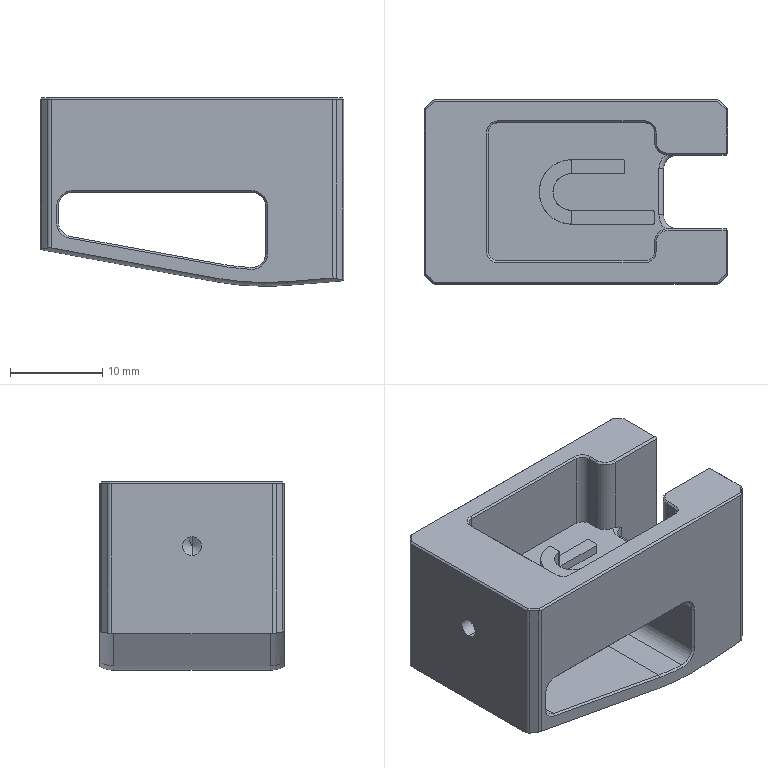NC program | NX | posted with a generic post | part box 33 x 20 x 20.478 mm
Lines 3457 to 5321 of 8500, first 1748 of 1863 lines:
(ZLEVEL_PROFILE_COPY , TOOL : D3)
N6882 T16 M6
N6884 G54
N6886 G17 G0 G90 X13.266 Y1.9 B0. C0. S9500 M3
N6888 G43 Z30. H16
N6890 Z0.301
N6892 G94 G1 Z-0.199 F1000.
N6894 X13.006 Y2.35
N6896 G3 X12.746 Y2.5 R0.3
N6898 G1 X11.
N6900 Y0.748
N6902 G3 X11.15 Y0.488 R0.3
N6904 G1 X11.6 Y0.228
N6906 Z0.301
N6908 G0 X13.266 Y1.9 Z0.102
N6910 G1 Z-0.398
N6912 X13.006 Y2.35
N6914 G3 X12.746 Y2.5 R0.3
N6916 G1 X11.
N6918 Y0.748
N6920 G3 X11.15 Y0.488 R0.3
N6922 G1 X11.6 Y0.228
N6924 Z0.102
N6926 G0 X13.266 Y1.9 Z-0.096
N6928 G1 Z-0.596
N6930 X13.006 Y2.35
N6932 G3 X12.746 Y2.5 R0.3
N6934 G1 X11.
N6936 Y0.748
N6938 G3 X11.15 Y0.488 R0.3
N6940 G1 X11.6 Y0.228
N6942 Z-0.096
N6944 G0 X13.266 Y1.9 Z-0.295
N6946 G1 Z-0.795
N6948 X13.006 Y2.35
N6950 G3 X12.746 Y2.5 R0.3
N6952 G1 X11.
N6954 Y0.748
N6956 G3 X11.15 Y0.488 R0.3
N6958 G1 X11.6 Y0.228
N6960 Z-0.295
N6962 G0 X13.266 Y1.9 Z-0.494
N6964 G1 Z-0.994
N6966 X13.006 Y2.35
N6968 G3 X12.746 Y2.5 R0.3
N6970 G1 X11.
N6972 Y0.748
N6974 G3 X11.15 Y0.488 R0.3
N6976 G1 X11.6 Y0.228
N6978 Z-0.494
N6980 G0 X13.266 Y1.9 Z-0.693
N6982 G1 Z-1.193
N6984 X13.006 Y2.35
N6986 G3 X12.746 Y2.5 R0.3
N6988 G1 X11.
N6990 Y0.748
N6992 G3 X11.15 Y0.488 R0.3
N6994 G1 X11.6 Y0.228
N6996 Z-0.693
N6998 G0 X13.266 Y1.9 Z-0.892
N7000 G1 Z-1.392
N7002 X13.006 Y2.35
N7004 G3 X12.746 Y2.5 R0.3
N7006 G1 X11.
N7008 Y0.748
N7010 G3 X11.15 Y0.488 R0.3
N7012 G1 X11.6 Y0.228
N7014 Z-0.892
N7016 G0 X13.266 Y1.9 Z-1.091
N7018 G1 Z-1.591
N7020 X13.006 Y2.35
N7022 G3 X12.746 Y2.5 R0.3
N7024 G1 X11.
N7026 Y0.748
N7028 G3 X11.15 Y0.488 R0.3
N7030 G1 X11.6 Y0.228
N7032 Z-1.091
N7034 G0 X13.266 Y1.9 Z-1.289
N7036 G1 Z-1.789
N7038 X13.006 Y2.35
N7040 G3 X12.746 Y2.5 R0.3
N7042 G1 X11.
N7044 Y0.748
N7046 G3 X11.15 Y0.488 R0.3
N7048 G1 X11.6 Y0.228
N7050 Z-1.289
N7052 G0 X13.266 Y1.9 Z-1.488
N7054 G1 Z-1.988
N7056 X13.006 Y2.35
N7058 G3 X12.746 Y2.5 R0.3
N7060 G1 X11.
N7062 Y0.748
N7064 G3 X11.15 Y0.488 R0.3
N7066 G1 X11.6 Y0.228
N7068 Z-1.488
N7070 G0 X13.266 Y1.9 Z-1.687
N7072 G1 Z-2.187
N7074 X13.006 Y2.35
N7076 G3 X12.746 Y2.5 R0.3
N7078 G1 X11.
N7080 Y0.748
N7082 G3 X11.15 Y0.488 R0.3
N7084 G1 X11.6 Y0.228
N7086 Z-1.687
N7088 G0 X13.266 Y1.9 Z-1.886
N7090 G1 Z-2.386
N7092 X13.006 Y2.35
N7094 G3 X12.746 Y2.5 R0.3
N7096 G1 X11.
N7098 Y0.748
N7100 G3 X11.15 Y0.488 R0.3
N7102 G1 X11.6 Y0.228
N7104 Z-1.886
N7106 G0 X13.266 Y1.9 Z-2.085
N7108 G1 Z-2.585
N7110 X13.006 Y2.35
N7112 G3 X12.746 Y2.5 R0.3
N7114 G1 X11.
N7116 Y0.748
N7118 G3 X11.15 Y0.488 R0.3
N7120 G1 X11.6 Y0.228
N7122 Z-2.085
N7124 G0 X13.266 Y1.9 Z-2.283
N7126 G1 Z-2.783
N7128 X13.006 Y2.35
N7130 G3 X12.746 Y2.5 R0.3
N7132 G1 X11.
N7134 Y0.748
N7136 G3 X11.15 Y0.488 R0.3
N7138 G1 X11.6 Y0.228
N7140 Z-2.283
N7142 G0 X13.266 Y1.9 Z-2.482
N7144 G1 Z-2.982
N7146 X13.006 Y2.35
N7148 G3 X12.746 Y2.5 R0.3
N7150 G1 X11.
N7152 Y0.748
N7154 G3 X11.15 Y0.488 R0.3
N7156 G1 X11.6 Y0.228
N7158 Z-2.482
N7160 G0 X13.266 Y1.9 Z-2.681
N7162 G1 Z-3.181
N7164 X13.006 Y2.35
N7166 G3 X12.746 Y2.5 R0.3
N7168 G1 X11.
N7170 Y0.748
N7172 G3 X11.15 Y0.488 R0.3
N7174 G1 X11.6 Y0.228
N7176 Z-2.681
N7178 G0 X13.266 Y1.9 Z-2.88
N7180 G1 Z-3.38
N7182 X13.006 Y2.35
N7184 G3 X12.746 Y2.5 R0.3
N7186 G1 X11.
N7188 Y0.748
N7190 G3 X11.15 Y0.488 R0.3
N7192 G1 X11.6 Y0.228
N7194 Z-2.88
N7196 G0 X13.266 Y1.9 Z-3.079
N7198 G1 Z-3.579
N7200 X13.006 Y2.35
N7202 G3 X12.746 Y2.5 R0.3
N7204 G1 X11.
N7206 Y0.748
N7208 G3 X11.15 Y0.488 R0.3
N7210 G1 X11.6 Y0.228
N7212 Z-3.079
N7214 G0 X13.266 Y1.9 Z-3.278
N7216 G1 Z-3.778
N7218 X13.006 Y2.35
N7220 G3 X12.746 Y2.5 R0.3
N7222 G1 X11.
N7224 Y0.748
N7226 G3 X11.15 Y0.488 R0.3
N7228 G1 X11.6 Y0.228
N7230 Z-3.278
N7232 G0 X13.266 Y1.9 Z-3.476
N7234 G1 Z-3.976
N7236 X13.006 Y2.35
N7238 G3 X12.746 Y2.5 R0.3
N7240 G1 X11.
N7242 Y0.748
N7244 G3 X11.15 Y0.488 R0.3
N7246 G1 X11.6 Y0.228
N7248 Z-3.476
N7250 G0 X13.266 Y1.9 Z-3.675
N7252 G1 Z-4.175
N7254 X13.006 Y2.35
N7256 G3 X12.746 Y2.5 R0.3
N7258 G1 X11.
N7260 Y0.748
N7262 G3 X11.15 Y0.488 R0.3
N7264 G1 X11.6 Y0.228
N7266 Z-3.675
N7268 G0 X13.266 Y1.9 Z-3.874
N7270 G1 Z-4.374
N7272 X13.006 Y2.35
N7274 G3 X12.746 Y2.5 R0.3
N7276 G1 X11.
N7278 Y0.748
N7280 G3 X11.15 Y0.488 R0.3
N7282 G1 X11.6 Y0.228
N7284 Z-3.874
N7286 G0 X13.266 Y1.9 Z-4.073
N7288 G1 Z-4.573
N7290 X13.006 Y2.35
N7292 G3 X12.746 Y2.5 R0.3
N7294 G1 X11.
N7296 Y0.748
N7298 G3 X11.15 Y0.488 R0.3
N7300 G1 X11.6 Y0.228
N7302 Z-4.073
N7304 G0 X13.266 Y1.9 Z-4.272
N7306 G1 Z-4.772
N7308 X13.006 Y2.35
N7310 G3 X12.746 Y2.5 R0.3
N7312 G1 X11.
N7314 Y0.748
N7316 G3 X11.15 Y0.488 R0.3
N7318 G1 X11.6 Y0.228
N7320 Z-4.272
N7322 G0 X13.266 Y1.9 Z-4.47
N7324 G1 Z-4.97
N7326 X13.006 Y2.35
N7328 G3 X12.746 Y2.5 R0.3
N7330 G1 X11.
N7332 Y0.748
N7334 G3 X11.15 Y0.488 R0.3
N7336 G1 X11.6 Y0.228
N7338 Z-4.47
N7340 G0 X13.266 Y1.9 Z-4.669
N7342 G1 Z-5.169
N7344 X13.006 Y2.35
N7346 G3 X12.746 Y2.5 R0.3
N7348 G1 X11.
N7350 Y0.748
N7352 G3 X11.15 Y0.488 R0.3
N7354 G1 X11.6 Y0.228
N7356 Z-4.669
N7358 G0 X13.266 Y1.9 Z-4.868
N7360 G1 Z-5.368
N7362 X13.006 Y2.35
N7364 G3 X12.746 Y2.5 R0.3
N7366 G1 X11.
N7368 Y0.748
N7370 G3 X11.15 Y0.488 R0.3
N7372 G1 X11.6 Y0.228
N7374 Z-4.868
N7376 G0 X13.266 Y1.9 Z-5.067
N7378 G1 Z-5.567
N7380 X13.006 Y2.35
N7382 G3 X12.746 Y2.5 R0.3
N7384 G1 X11.
N7386 Y0.748
N7388 G3 X11.15 Y0.488 R0.3
N7390 G1 X11.6 Y0.228
N7392 Z-5.067
N7394 G0 X13.266 Y1.9 Z-5.266
N7396 G1 Z-5.766
N7398 X13.006 Y2.35
N7400 G3 X12.746 Y2.5 R0.3
N7402 G1 X11.
N7404 Y0.748
N7406 G3 X11.15 Y0.488 R0.3
N7408 G1 X11.6 Y0.228
N7410 Z-5.266
N7412 G0 X13.266 Y1.9 Z-5.465
N7414 G1 Z-5.965
N7416 X13.006 Y2.35
N7418 G3 X12.746 Y2.5 R0.3
N7420 G1 X11.
N7422 Y0.748
N7424 G3 X11.15 Y0.488 R0.3
N7426 G1 X11.6 Y0.228
N7428 Z-5.465
N7430 G0 X13.266 Y1.9 Z-5.663
N7432 G1 Z-6.163
N7434 X13.006 Y2.35
N7436 G3 X12.746 Y2.5 R0.3
N7438 G1 X11.
N7440 Y0.748
N7442 G3 X11.15 Y0.488 R0.3
N7444 G1 X11.6 Y0.228
N7446 Z-5.663
N7448 G0 X13.266 Y1.9 Z-5.862
N7450 G1 Z-6.362
N7452 X13.006 Y2.35
N7454 G3 X12.747 Y2.5 R0.3
N7456 G1 X11.
N7458 Y0.748
N7460 G3 X11.15 Y0.488 R0.3
N7462 G1 X11.6 Y0.228
N7464 Z-5.862
N7466 G0 X13.266 Y1.9 Z-6.061
N7468 G1 Z-6.561
N7470 X13.006 Y2.35
N7472 G3 X12.747 Y2.5 R0.3
N7474 G1 X11.
N7476 Y0.748
N7478 G3 X11.15 Y0.488 R0.3
N7480 G1 X11.6 Y0.228
N7482 Z-6.061
N7484 G0 X13.266 Y1.9 Z-6.26
N7486 G1 Z-6.76
N7488 X13.006 Y2.35
N7490 G3 X12.747 Y2.5 R0.3
N7492 G1 X11.
N7494 Y0.748
N7496 G3 X11.15 Y0.488 R0.3
N7498 G1 X11.6 Y0.228
N7500 Z-6.26
N7502 G0 X13.266 Y1.9 Z-6.459
N7504 G1 Z-6.959
N7506 X13.006 Y2.35
N7508 G3 X12.747 Y2.5 R0.3
N7510 G1 X11.
N7512 Y0.748
N7514 G3 X11.15 Y0.488 R0.3
N7516 G1 X11.6 Y0.228
N7518 Z-6.459
N7520 G0 X13.266 Y1.9 Z-6.657
N7522 G1 Z-7.157
N7524 X13.006 Y2.35
N7526 G3 X12.747 Y2.5 R0.3
N7528 G1 X11.
N7530 Y0.748
N7532 G3 X11.15 Y0.488 R0.3
N7534 G1 X11.6 Y0.228
N7536 Z-6.657
N7538 G0 X13.266 Y1.9 Z-6.856
N7540 G1 Z-7.356
N7542 X13.006 Y2.35
N7544 G3 X12.747 Y2.5 R0.3
N7546 G1 X11.
N7548 Y0.748
N7550 G3 X11.15 Y0.488 R0.3
N7552 G1 X11.6 Y0.228
N7554 Z-6.856
N7556 G0 X13.266 Y1.9 Z-7.055
N7558 G1 Z-7.555
N7560 X13.006 Y2.35
N7562 G3 X12.747 Y2.5 R0.3
N7564 G1 X11.
N7566 Y0.748
N7568 G3 X11.15 Y0.488 R0.3
N7570 G1 X11.6 Y0.228
N7572 Z-7.055
N7574 G0 X13.266 Y1.9 Z-7.254
N7576 G1 Z-7.754
N7578 X13.006 Y2.35
N7580 G3 X12.747 Y2.5 R0.3
N7582 G1 X11.
N7584 Y0.748
N7586 G3 X11.15 Y0.488 R0.3
N7588 G1 X11.6 Y0.228
N7590 Z-7.254
N7592 G0 X13.266 Y1.9 Z-7.453
N7594 G1 Z-7.953
N7596 X13.006 Y2.35
N7598 G3 X12.747 Y2.5 R0.3
N7600 G1 X11.
N7602 Y0.748
N7604 G3 X11.15 Y0.488 R0.3
N7606 G1 X11.6 Y0.228
N7608 Z-7.453
N7610 G0 X13.266 Y1.9 Z-7.652
N7612 G1 Z-8.152
N7614 X13.006 Y2.35
N7616 G3 X12.747 Y2.5 R0.3
N7618 G1 X11.
N7620 Y0.748
N7622 G3 X11.15 Y0.488 R0.3
N7624 G1 X11.6 Y0.228
N7626 Z-7.652
N7628 G0 X13.266 Y1.9 Z-7.85
N7630 G1 Z-8.35
N7632 X13.006 Y2.35
N7634 G3 X12.747 Y2.5 R0.3
N7636 G1 X11.
N7638 Y0.748
N7640 G3 X11.15 Y0.488 R0.3
N7642 G1 X11.6 Y0.228
N7644 Z-7.85
N7646 G0 X13.266 Y1.9 Z-8.049
N7648 G1 Z-8.549
N7650 X13.006 Y2.35
N7652 G3 X12.747 Y2.5 R0.3
N7654 G1 X11.
N7656 Y0.748
N7658 G3 X11.15 Y0.488 R0.3
N7660 G1 X11.6 Y0.228
N7662 Z-8.049
N7664 G0 X13.266 Y1.9 Z-8.248
N7666 G1 Z-8.748
N7668 X13.006 Y2.35
N7670 G3 X12.747 Y2.5 R0.3
N7672 G1 X11.
N7674 Y0.748
N7676 G3 X11.15 Y0.488 R0.3
N7678 G1 X11.6 Y0.228
N7680 Z-8.248
N7682 G0 X13.266 Y1.9 Z-8.447
N7684 G1 Z-8.947
N7686 X13.006 Y2.35
N7688 G3 X12.747 Y2.5 R0.3
N7690 G1 X11.
N7692 Y0.748
N7694 G3 X11.15 Y0.488 R0.3
N7696 G1 X11.6 Y0.228
N7698 Z-8.447
N7700 G0 X13.266 Y1.9 Z-8.646
N7702 G1 Z-9.146
N7704 X13.006 Y2.35
N7706 G3 X12.747 Y2.5 R0.3
N7708 G1 X11.
N7710 Y0.748
N7712 G3 X11.15 Y0.488 R0.3
N7714 G1 X11.6 Y0.228
N7716 Z-8.646
N7718 G0 X13.266 Y1.9 Z-8.844
N7720 G1 Z-9.344
N7722 X13.006 Y2.35
N7724 G3 X12.747 Y2.5 R0.3
N7726 G1 X11.
N7728 Y0.748
N7730 G3 X11.15 Y0.488 R0.3
N7732 G1 X11.6 Y0.228
N7734 Z-8.844
N7736 G0 X13.266 Y1.9 Z-9.043
N7738 G1 Z-9.543
N7740 X13.006 Y2.35
N7742 G3 X12.747 Y2.5 R0.3
N7744 G1 X11.
N7746 Y0.748
N7748 G3 X11.15 Y0.488 R0.3
N7750 G1 X11.6 Y0.228
N7752 Z-9.043
N7754 G0 X13.266 Y1.9 Z-9.242
N7756 G1 Z-9.742
N7758 X13.006 Y2.35
N7760 G3 X12.747 Y2.5 R0.3
N7762 G1 X11.
N7764 Y0.748
N7766 G3 X11.15 Y0.488 R0.3
N7768 G1 X11.6 Y0.228
N7770 Z-9.242
N7772 G0 X13.266 Y1.9 Z-9.441
N7774 G1 Z-9.941
N7776 X13.006 Y2.35
N7778 G3 X12.747 Y2.5 R0.3
N7780 G1 X11.
N7782 Y0.748
N7784 G3 X11.15 Y0.488 R0.3
N7786 G1 X11.6 Y0.228
N7788 Z-9.441
N7790 G0 X13.266 Y1.9 Z-9.64
N7792 G1 Z-10.14
N7794 X13.006 Y2.35
N7796 G3 X12.747 Y2.5 R0.3
N7798 G1 X11.
N7800 Y0.748
N7802 G3 X11.15 Y0.488 R0.3
N7804 G1 X11.6 Y0.228
N7806 Z-9.64
N7808 G0 X13.266 Y1.9 Z-9.839
N7810 G1 Z-10.339
N7812 X13.006 Y2.35
N7814 G3 X12.747 Y2.5 R0.3
N7816 G1 X11.
N7818 Y0.748
N7820 G3 X11.15 Y0.488 R0.3
N7822 G1 X11.6 Y0.228
N7824 Z-9.839
N7826 G0 X13.266 Y1.9 Z-10.037
N7828 G1 Z-10.537
N7830 X13.006 Y2.35
N7832 G3 X12.747 Y2.5 R0.3
N7834 G1 X11.
N7836 Y0.748
N7838 G3 X11.15 Y0.488 R0.3
N7840 G1 X11.6 Y0.228
N7842 Z-10.037
N7844 G0 X13.266 Y1.9 Z-10.236
N7846 G1 Z-10.736
N7848 X13.006 Y2.35
N7850 G3 X12.747 Y2.5 R0.3
N7852 G1 X11.
N7854 Y0.748
N7856 G3 X11.15 Y0.488 R0.3
N7858 G1 X11.6 Y0.228
N7860 Z-10.236
N7862 G0 X13.266 Y1.9 Z-10.435
N7864 G1 Z-10.935
N7866 X13.006 Y2.35
N7868 G3 X12.747 Y2.5 R0.3
N7870 G1 X11.
N7872 Y0.748
N7874 G3 X11.15 Y0.488 R0.3
N7876 G1 X11.6 Y0.228
N7878 Z-10.435
N7880 G0 X13.266 Y1.9 Z-10.634
N7882 G1 Z-11.134
N7884 X13.006 Y2.35
N7886 G3 X12.747 Y2.5 R0.3
N7888 G1 X11.
N7890 Y0.748
N7892 G3 X11.15 Y0.488 R0.3
N7894 G1 X11.6 Y0.228
N7896 Z-10.634
N7898 G0 X13.266 Y1.9 Z-10.833
N7900 G1 Z-11.333
N7902 X13.006 Y2.35
N7904 G3 X12.747 Y2.5 R0.3
N7906 G1 X11.
N7908 Y0.748
N7910 G3 X11.15 Y0.488 R0.3
N7912 G1 X11.6 Y0.228
N7914 Z-10.833
N7916 G0 X13.266 Y1.9 Z-11.031
N7918 G1 Z-11.531
N7920 X13.006 Y2.35
N7922 G3 X12.747 Y2.5 R0.3
N7924 G1 X11.
N7926 Y0.748
N7928 G3 X11.15 Y0.488 R0.3
N7930 G1 X11.6 Y0.228
N7932 Z-11.031
N7934 G0 X13.266 Y1.9 Z-11.23
N7936 G1 Z-11.73
N7938 X13.006 Y2.35
N7940 G3 X12.747 Y2.5 R0.3
N7942 G1 X11.
N7944 Y0.748
N7946 G3 X11.15 Y0.488 R0.3
N7948 G1 X11.6 Y0.228
N7950 Z-11.23
N7952 G0 X13.266 Y1.9 Z-11.429
N7954 G1 Z-11.929
N7956 X13.006 Y2.35
N7958 G3 X12.747 Y2.5 R0.3
N7960 G1 X11.
N7962 Y0.748
N7964 G3 X11.15 Y0.488 R0.3
N7966 G1 X11.6 Y0.228
N7968 Z-11.429
N7970 G0 X13.266 Y1.9 Z-11.628
N7972 G1 Z-12.128
N7974 X13.006 Y2.35
N7976 G3 X12.747 Y2.5 R0.3
N7978 G1 X11.
N7980 Y0.748
N7982 G3 X11.15 Y0.488 R0.3
N7984 G1 X11.6 Y0.228
N7986 Z-11.628
N7988 G0 X13.266 Y1.9 Z-11.827
N7990 G1 Z-12.327
N7992 X13.006 Y2.35
N7994 G3 X12.747 Y2.5 R0.3
N7996 G1 X11.
N7998 Y0.748
N8000 G3 X11.15 Y0.488 R0.3
N8002 G1 X11.6 Y0.228
N8004 Z-11.827
N8006 G0 X13.266 Y1.9 Z-12.026
N8008 G1 Z-12.526
N8010 X13.006 Y2.35
N8012 G3 X12.747 Y2.5 R0.3
N8014 G1 X11.
N8016 Y0.748
N8018 G3 X11.15 Y0.488 R0.3
N8020 G1 X11.6 Y0.228
N8022 Z-12.026
N8024 G0 X13.266 Y1.9 Z-12.224
N8026 G1 Z-12.724
N8028 X13.006 Y2.35
N8030 G3 X12.747 Y2.5 R0.3
N8032 G1 X11.
N8034 Y0.748
N8036 G3 X11.15 Y0.488 R0.3
N8038 G1 X11.6 Y0.228
N8040 Z-12.224
N8042 G0 X13.266 Y1.9 Z-12.423
N8044 G1 Z-12.923
N8046 X13.006 Y2.35
N8048 G3 X12.747 Y2.5 R0.3
N8050 G1 X11.
N8052 Y0.748
N8054 G3 X11.15 Y0.488 R0.3
N8056 G1 X11.6 Y0.228
N8058 Z-12.423
N8060 G0 X13.266 Y1.9 Z-12.622
N8062 G1 Z-13.122
N8064 X13.006 Y2.35
N8066 G3 X12.747 Y2.5 R0.3
N8068 G1 X11.
N8070 Y0.748
N8072 G3 X11.15 Y0.488 R0.3
N8074 G1 X11.6 Y0.228
N8076 Z-12.622
N8078 G0 X13.266 Y1.9 Z-12.821
N8080 G1 Z-13.321
N8082 X13.006 Y2.35
N8084 G3 X12.747 Y2.5 R0.3
N8086 G1 X11.
N8088 Y0.748
N8090 G3 X11.15 Y0.488 R0.3
N8092 G1 X11.6 Y0.228
N8094 Z-12.821
N8096 G0 X13.266 Y1.9 Z-13.02
N8098 G1 Z-13.52
N8100 X13.006 Y2.35
N8102 G3 X12.747 Y2.5 R0.3
N8104 G1 X11.
N8106 Y0.748
N8108 G3 X11.15 Y0.488 R0.3
N8110 G1 X11.6 Y0.228
N8112 Z-13.02
N8114 G0 X13.266 Y1.9 Z-13.218
N8116 G1 Z-13.718
N8118 X13.006 Y2.35
N8120 G3 X12.747 Y2.5 R0.3
N8122 G1 X11.
N8124 Y0.748
N8126 G3 X11.15 Y0.488 R0.3
N8128 G1 X11.6 Y0.228
N8130 Z-13.218
N8132 G0 X13.266 Y1.9 Z-13.417
N8134 G1 Z-13.917
N8136 X13.006 Y2.35
N8138 G3 X12.747 Y2.5 R0.3
N8140 G1 X11.
N8142 Y0.748
N8144 G3 X11.15 Y0.488 R0.3
N8146 G1 X11.6 Y0.228
N8148 Z-13.417
N8150 G0 X13.266 Y1.9 Z-13.616
N8152 G1 Z-14.116
N8154 X13.006 Y2.35
N8156 G3 X12.747 Y2.5 R0.3
N8158 G1 X11.
N8160 Y0.748
N8162 G3 X11.15 Y0.488 R0.3
N8164 G1 X11.6 Y0.228
N8166 Z-13.616
N8168 G0 X13.266 Y1.9 Z-13.815
N8170 G1 Z-14.315
N8172 X13.006 Y2.35
N8174 G3 X12.747 Y2.5 R0.3
N8176 G1 X11.
N8178 Y0.748
N8180 G3 X11.15 Y0.488 R0.3
N8182 G1 X11.6 Y0.228
N8184 Z-13.815
N8186 G0 X13.266 Y1.9 Z-14.014
N8188 G1 Z-14.514
N8190 X13.006 Y2.35
N8192 G3 X12.747 Y2.5 R0.3
N8194 G1 X11.
N8196 Y0.748
N8198 G3 X11.15 Y0.488 R0.3
N8200 G1 X11.6 Y0.228
N8202 Z-14.014
N8204 G0 X13.266 Y1.9 Z-14.213
N8206 G1 Z-14.713
N8208 X13.006 Y2.35
N8210 G3 X12.747 Y2.5 R0.3
N8212 G1 X11.
N8214 Y0.748
N8216 G3 X11.15 Y0.488 R0.3
N8218 G1 X11.6 Y0.228
N8220 Z-14.213
N8222 G0 X13.266 Y1.9 Z-14.411
N8224 G1 Z-14.911
N8226 X13.006 Y2.35
N8228 G3 X12.747 Y2.5 R0.3
N8230 G1 X11.
N8232 Y0.748
N8234 G3 X11.15 Y0.488 R0.3
N8236 G1 X11.6 Y0.228
N8238 Z-14.411
N8240 G0 X13.266 Y1.9 Z-14.61
N8242 G1 Z-15.11
N8244 X13.006 Y2.35
N8246 G3 X12.747 Y2.5 R0.3
N8248 G1 X11.
N8250 Y0.748
N8252 G3 X11.15 Y0.488 R0.3
N8254 G1 X11.6 Y0.228
N8256 Z-14.61
N8258 G0 X13.266 Y1.9 Z-14.809
N8260 G1 Z-15.309
N8262 X13.006 Y2.35
N8264 G3 X12.747 Y2.5 R0.3
N8266 G1 X11.
N8268 Y0.748
N8270 G3 X11.15 Y0.488 R0.3
N8272 G1 X11.6 Y0.228
N8274 Z-14.809
N8276 G0 X13.266 Y1.9 Z-15.008
N8278 G1 Z-15.508
N8280 X13.006 Y2.35
N8282 G3 X12.747 Y2.5 R0.3
N8284 G1 X11.
N8286 Y0.748
N8288 G3 X11.15 Y0.488 R0.3
N8290 G1 X11.6 Y0.228
N8292 Z-15.008
N8294 G0 X13.266 Y1.9 Z-15.207
N8296 G1 Z-15.707
N8298 X13.006 Y2.35
N8300 G3 X12.747 Y2.5 R0.3
N8302 G1 X11.
N8304 Y0.748
N8306 G3 X11.15 Y0.488 R0.3
N8308 G1 X11.6 Y0.228
N8310 Z-15.207
N8312 G0 X13.266 Y1.9 Z-15.405
N8314 G1 Z-15.905
N8316 X13.006 Y2.35
N8318 G3 X12.747 Y2.5 R0.3
N8320 G1 X11.
N8322 Y0.748
N8324 G3 X11.15 Y0.488 R0.3
N8326 G1 X11.6 Y0.228
N8328 Z-15.405
N8330 G0 X13.266 Y1.9 Z-15.604
N8332 G1 Z-16.104
N8334 X13.006 Y2.35
N8336 G3 X12.747 Y2.5 R0.3
N8338 G1 X11.
N8340 Y0.748
N8342 G3 X11.15 Y0.488 R0.3
N8344 G1 X11.6 Y0.228
N8346 Z-15.604
N8348 G0 X13.266 Y1.9 Z-15.803
N8350 G1 Z-16.303
N8352 X13.006 Y2.35
N8354 G3 X12.747 Y2.5 R0.3
N8356 G1 X11.
N8358 Y0.748
N8360 G3 X11.15 Y0.488 R0.3
N8362 G1 X11.6 Y0.228
N8364 Z-15.803
N8366 G0 X13.266 Y1.9 Z-16.002
N8368 G1 Z-16.502
N8370 X13.006 Y2.35
N8372 G3 X12.747 Y2.5 R0.3
N8374 G1 X11.
N8376 Y0.748
N8378 G3 X11.15 Y0.488 R0.3
N8380 G1 X11.6 Y0.228
N8382 Z-16.002
N8384 G0 X13.266 Y1.9 Z-16.201
N8386 G1 Z-16.701
N8388 X13.006 Y2.35
N8390 G3 X12.747 Y2.5 R0.3
N8392 G1 X11.
N8394 Y0.748
N8396 G3 X11.15 Y0.488 R0.3
N8398 G1 X11.6 Y0.228
N8400 Z-16.201
N8402 G0 X13.266 Y1.9 Z-16.4
N8404 G1 Z-16.9
N8406 X13.006 Y2.35
N8408 G3 X12.747 Y2.5 R0.3
N8410 G1 X11.
N8412 Y0.748
N8414 G3 X11.15 Y0.488 R0.3
N8416 G1 X11.6 Y0.228
N8418 Z-16.4
N8420 G0 X13.266 Y1.9 Z-16.598
N8422 G1 Z-17.098
N8424 X13.006 Y2.35
N8426 G3 X12.747 Y2.5 R0.3
N8428 G1 X11.
N8430 Y0.748
N8432 G3 X11.15 Y0.488 R0.3
N8434 G1 X11.6 Y0.228
N8436 Z-16.598
N8438 G0 X13.266 Y1.9 Z-16.797
N8440 G1 Z-17.297
N8442 X13.006 Y2.35
N8444 G3 X12.747 Y2.5 R0.3
N8446 G1 X11.
N8448 Y0.748
N8450 G3 X11.15 Y0.488 R0.3
N8452 G1 X11.6 Y0.228
N8454 Z-16.797
N8456 G0 X13.266 Y1.9 Z-16.996
N8458 G1 Z-17.496
N8460 X13.006 Y2.35
N8462 G3 X12.747 Y2.5 R0.3
N8464 G1 X11.
N8466 Y0.748
N8468 G3 X11.15 Y0.488 R0.3
N8470 G1 X11.6 Y0.228
N8472 Z-16.996
N8474 G0 X13.266 Y1.9 Z-17.195
N8476 G1 Z-17.695
N8478 X13.006 Y2.35
N8480 G3 X12.747 Y2.5 R0.3
N8482 G1 X11.
N8484 Y0.748
N8486 G3 X11.15 Y0.488 R0.3
N8488 G1 X11.6 Y0.228
N8490 Z-17.195
N8492 G0 X13.266 Y1.9 Z-17.394
N8494 G1 Z-17.894
N8496 X13.006 Y2.35
N8498 G3 X12.747 Y2.5 R0.3
N8500 G1 X11.
N8502 Y0.748
N8504 G3 X11.15 Y0.488 R0.3
N8506 G1 X11.6 Y0.228
N8508 Z-17.394
N8510 G0 X13.266 Y1.9 Z-17.592
N8512 G1 Z-18.092
N8514 X13.006 Y2.35
N8516 G3 X12.747 Y2.5 R0.3
N8518 G1 X11.
N8520 Y0.748
N8522 G3 X11.15 Y0.488 R0.3
N8524 G1 X11.6 Y0.228
N8526 Z-17.592
N8528 G0 X13.266 Y1.9 Z-17.791
N8530 G1 Z-18.291
N8532 X13.006 Y2.35
N8534 G3 X12.747 Y2.5 R0.3
N8536 G1 X11.
N8538 Y0.748
N8540 G3 X11.15 Y0.488 R0.3
N8542 G1 X11.6 Y0.228
N8544 Z-17.791
N8546 G0 X13.266 Y1.9 Z-17.99
N8548 G1 Z-18.49
N8550 X13.006 Y2.35
N8552 G3 X12.747 Y2.5 R0.3
N8554 G1 X11.
N8556 Y0.748
N8558 G3 X11.15 Y0.488 R0.3
N8560 G1 X11.6 Y0.228
N8562 Z-17.99
N8564 G0 X13.266 Y1.9 Z-18.189
N8566 G1 Z-18.689
N8568 X13.006 Y2.35
N8570 G3 X12.747 Y2.5 R0.3
N8572 G1 X11.
N8574 Y0.748
N8576 G3 X11.15 Y0.488 R0.3
N8578 G1 X11.6 Y0.228
N8580 Z-18.189
N8582 G0 X13.266 Y1.9 Z-18.388
N8584 G1 Z-18.888
N8586 X13.006 Y2.35
N8588 G3 X12.747 Y2.5 R0.3
N8590 G1 X11.
N8592 Y0.748
N8594 G3 X11.15 Y0.488 R0.3
N8596 G1 X11.6 Y0.228
N8598 Z-18.388
N8600 G0 X13.266 Y1.9 Z-18.587
N8602 G1 Z-19.087
N8604 X13.006 Y2.35
N8606 G3 X12.747 Y2.5 R0.3
N8608 G1 X11.
N8610 Y0.748
N8612 G3 X11.15 Y0.488 R0.3
N8614 G1 X11.6 Y0.228
N8616 Z-18.587
N8618 G0 X13.266 Y1.9 Z-18.785
N8620 G1 Z-19.285
N8622 X13.006 Y2.35
N8624 G3 X12.747 Y2.5 R0.3
N8626 G1 X11.
N8628 Y0.748
N8630 G3 X11.15 Y0.488 R0.3
N8632 G1 X11.6 Y0.228
N8634 Z-18.785
N8636 G0 X13.266 Y1.9 Z-18.984
N8638 G1 Z-19.484
N8640 X13.006 Y2.35
N8642 G3 X12.747 Y2.5 R0.3
N8644 G1 X11.
N8646 Y0.748
N8648 G3 X11.15 Y0.488 R0.3
N8650 G1 X11.6 Y0.228
N8652 Z-18.984
N8654 G0 X13.266 Y1.9 Z-19.183
N8656 G1 Z-19.683
N8658 X13.006 Y2.35
N8660 G3 X12.747 Y2.5 R0.3
N8662 G1 X11.
N8664 Y0.748
N8666 G3 X11.15 Y0.488 R0.3
N8668 G1 X11.6 Y0.228
N8670 Z-19.183
N8672 G0 X13.266 Y1.9 Z-19.382
N8674 G1 Z-19.882
N8676 X13.006 Y2.35
N8678 G3 X12.747 Y2.5 R0.3
N8680 G1 X11.
N8682 Y0.748
N8684 G3 X11.15 Y0.488 R0.3
N8686 G1 X11.6 Y0.228
N8688 Z-19.382
N8690 G0 X13.266 Y1.9 Z-19.581
N8692 G1 Z-20.081
N8694 X13.006 Y2.35
N8696 G3 X12.747 Y2.5 R0.3
N8698 G1 X11.
N8700 Y0.748
N8702 G3 X11.15 Y0.488 R0.3
N8704 G1 X11.6 Y0.228
N8706 Z-19.581
N8708 G0 X13.266 Y1.9 Z-19.78
N8710 G1 Z-20.28
N8712 X13.006 Y2.35
N8714 G3 X12.747 Y2.5 R0.3
N8716 G1 X11.
N8718 Y0.748
N8720 G3 X11.15 Y0.488 R0.3
N8722 G1 X11.6 Y0.228
N8724 Z-19.78
N8726 G0 X13.266 Y1.9 Z-19.978
N8728 G1 Z-20.478
N8730 X13.006 Y2.35
N8732 G3 X12.747 Y2.5 R0.3
N8734 G1 X11.
N8736 Y0.748
N8738 G3 X11.15 Y0.488 R0.3
N8740 G1 X11.6 Y0.228
N8742 Z-19.978
N8744 G0 Z30.
N8746 Y-0.226
N8748 Z0.301
N8750 G1 Z-0.199
N8752 X11.15 Y-0.486
N8754 G3 X11. Y-0.746 R0.3
N8756 G1 Y-2.5
N8758 X12.754
N8760 G3 X13.014 Y-2.35 R0.3
N8762 G1 X13.274 Y-1.9
N8764 Z0.301
N8766 G0 X11.6 Y-0.226 Z0.102
N8768 G1 Z-0.398
N8770 X11.15 Y-0.486
N8772 G3 X11. Y-0.746 R0.3
N8774 G1 Y-2.5
N8776 X12.754
N8778 G3 X13.014 Y-2.35 R0.3
N8780 G1 X13.274 Y-1.9
N8782 Z0.102
N8784 G0 X11.6 Y-0.226 Z-0.096
N8786 G1 Z-0.596
N8788 X11.15 Y-0.486
N8790 G3 X11. Y-0.746 R0.3
N8792 G1 Y-2.5
N8794 X12.754
N8796 G3 X13.014 Y-2.35 R0.3
N8798 G1 X13.274 Y-1.9
N8800 Z-0.096
N8802 G0 X11.6 Y-0.226 Z-0.295
N8804 G1 Z-0.795
N8806 X11.15 Y-0.486
N8808 G3 X11. Y-0.746 R0.3
N8810 G1 Y-2.5
N8812 X12.754
N8814 G3 X13.014 Y-2.35 R0.3
N8816 G1 X13.274 Y-1.9
N8818 Z-0.295
N8820 G0 X11.6 Y-0.226 Z-0.494
N8822 G1 Z-0.994
N8824 X11.15 Y-0.486
N8826 G3 X11. Y-0.746 R0.3
N8828 G1 Y-2.5
N8830 X12.754
N8832 G3 X13.014 Y-2.35 R0.3
N8834 G1 X13.274 Y-1.9
N8836 Z-0.494
N8838 G0 X11.6 Y-0.226 Z-0.693
N8840 G1 Z-1.193
N8842 X11.15 Y-0.486
N8844 G3 X11. Y-0.746 R0.3
N8846 G1 Y-2.5
N8848 X12.754
N8850 G3 X13.014 Y-2.35 R0.3
N8852 G1 X13.274 Y-1.9
N8854 Z-0.693
N8856 G0 X11.6 Y-0.226 Z-0.892
N8858 G1 Z-1.392
N8860 X11.15 Y-0.486
N8862 G3 X11. Y-0.746 R0.3
N8864 G1 Y-2.5
N8866 X12.754
N8868 G3 X13.014 Y-2.35 R0.3
N8870 G1 X13.274 Y-1.9
N8872 Z-0.892
N8874 G0 X11.6 Y-0.226 Z-1.091
N8876 G1 Z-1.591
N8878 X11.15 Y-0.486
N8880 G3 X11. Y-0.746 R0.3
N8882 G1 Y-2.5
N8884 X12.754
N8886 G3 X13.014 Y-2.35 R0.3
N8888 G1 X13.274 Y-1.9
N8890 Z-1.091
N8892 G0 X11.6 Y-0.226 Z-1.289
N8894 G1 Z-1.789
N8896 X11.15 Y-0.486
N8898 G3 X11. Y-0.746 R0.3
N8900 G1 Y-2.5
N8902 X12.754
N8904 G3 X13.014 Y-2.35 R0.3
N8906 G1 X13.274 Y-1.9
N8908 Z-1.289
N8910 G0 X11.6 Y-0.226 Z-1.488
N8912 G1 Z-1.988
N8914 X11.15 Y-0.486
N8916 G3 X11. Y-0.746 R0.3
N8918 G1 Y-2.5
N8920 X12.754
N8922 G3 X13.014 Y-2.35 R0.3
N8924 G1 X13.274 Y-1.9
N8926 Z-1.488
N8928 G0 X11.6 Y-0.226 Z-1.687
N8930 G1 Z-2.187
N8932 X11.15 Y-0.486
N8934 G3 X11. Y-0.746 R0.3
N8936 G1 Y-2.5
N8938 X12.754
N8940 G3 X13.014 Y-2.35 R0.3
N8942 G1 X13.274 Y-1.9
N8944 Z-1.687
N8946 G0 X11.6 Y-0.226 Z-1.886
N8948 G1 Z-2.386
N8950 X11.15 Y-0.486
N8952 G3 X11. Y-0.746 R0.3
N8954 G1 Y-2.5
N8956 X12.754
N8958 G3 X13.014 Y-2.35 R0.3
N8960 G1 X13.274 Y-1.9
N8962 Z-1.886
N8964 G0 X11.6 Y-0.226 Z-2.085
N8966 G1 Z-2.585
N8968 X11.15 Y-0.486
N8970 G3 X11. Y-0.746 R0.3
N8972 G1 Y-2.5
N8974 X12.754
N8976 G3 X13.014 Y-2.35 R0.3
N8978 G1 X13.274 Y-1.9
N8980 Z-2.085
N8982 G0 X11.6 Y-0.226 Z-2.283
N8984 G1 Z-2.783
N8986 X11.15 Y-0.486
N8988 G3 X11. Y-0.746 R0.3
N8990 G1 Y-2.5
N8992 X12.754
N8994 G3 X13.014 Y-2.35 R0.3
N8996 G1 X13.274 Y-1.9
N8998 Z-2.283
N9000 G0 X11.6 Y-0.226 Z-2.482
N9002 G1 Z-2.982
N9004 X11.15 Y-0.486
N9006 G3 X11. Y-0.746 R0.3
N9008 G1 Y-2.5
N9010 X12.754
N9012 G3 X13.014 Y-2.35 R0.3
N9014 G1 X13.274 Y-1.9
N9016 Z-2.482
N9018 G0 X11.6 Y-0.226 Z-2.681
N9020 G1 Z-3.181
N9022 X11.15 Y-0.486
N9024 G3 X11. Y-0.746 R0.3
N9026 G1 Y-2.5
N9028 X12.754
N9030 G3 X13.014 Y-2.35 R0.3
N9032 G1 X13.274 Y-1.9
N9034 Z-2.681
N9036 G0 X11.6 Y-0.226 Z-2.88
N9038 G1 Z-3.38
N9040 X11.15 Y-0.486
N9042 G3 X11. Y-0.746 R0.3
N9044 G1 Y-2.5
N9046 X12.754
N9048 G3 X13.014 Y-2.35 R0.3
N9050 G1 X13.274 Y-1.9
N9052 Z-2.88
N9054 G0 X11.6 Y-0.226 Z-3.079
N9056 G1 Z-3.579
N9058 X11.15 Y-0.486
N9060 G3 X11. Y-0.746 R0.3
N9062 G1 Y-2.5
N9064 X12.754
N9066 G3 X13.014 Y-2.35 R0.3
N9068 G1 X13.274 Y-1.9
N9070 Z-3.079
N9072 G0 X11.6 Y-0.226 Z-3.278
N9074 G1 Z-3.778
N9076 X11.15 Y-0.486
N9078 G3 X11. Y-0.746 R0.3
N9080 G1 Y-2.5
N9082 X12.754
N9084 G3 X13.014 Y-2.35 R0.3
N9086 G1 X13.274 Y-1.9
N9088 Z-3.278
N9090 G0 X11.6 Y-0.226 Z-3.476
N9092 G1 Z-3.976
N9094 X11.15 Y-0.486
N9096 G3 X11. Y-0.746 R0.3
N9098 G1 Y-2.5
N9100 X12.754
N9102 G3 X13.014 Y-2.35 R0.3
N9104 G1 X13.274 Y-1.9
N9106 Z-3.476
N9108 G0 X11.6 Y-0.226 Z-3.675
N9110 G1 Z-4.175
N9112 X11.15 Y-0.486
N9114 G3 X11. Y-0.746 R0.3
N9116 G1 Y-2.5
N9118 X12.754
N9120 G3 X13.014 Y-2.35 R0.3
N9122 G1 X13.274 Y-1.9
N9124 Z-3.675
N9126 G0 X11.6 Y-0.226 Z-3.874
N9128 G1 Z-4.374
N9130 X11.15 Y-0.486
N9132 G3 X11. Y-0.746 R0.3
N9134 G1 Y-2.5
N9136 X12.754
N9138 G3 X13.014 Y-2.35 R0.3
N9140 G1 X13.274 Y-1.9
N9142 Z-3.874
N9144 G0 X11.6 Y-0.226 Z-4.073
N9146 G1 Z-4.573
N9148 X11.15 Y-0.486
N9150 G3 X11. Y-0.746 R0.3
N9152 G1 Y-2.5
N9154 X12.754
N9156 G3 X13.014 Y-2.35 R0.3
N9158 G1 X13.274 Y-1.9
N9160 Z-4.073
N9162 G0 X11.6 Y-0.226 Z-4.272
N9164 G1 Z-4.772
N9166 X11.15 Y-0.486
N9168 G3 X11. Y-0.746 R0.3
N9170 G1 Y-2.5
N9172 X12.754
N9174 G3 X13.014 Y-2.35 R0.3
N9176 G1 X13.274 Y-1.9
N9178 Z-4.272
N9180 G0 X11.6 Y-0.226 Z-4.47
N9182 G1 Z-4.97
N9184 X11.15 Y-0.486
N9186 G3 X11. Y-0.746 R0.3
N9188 G1 Y-2.5
N9190 X12.754
N9192 G3 X13.014 Y-2.35 R0.3
N9194 G1 X13.274 Y-1.9
N9196 Z-4.47
N9198 G0 X11.6 Y-0.226 Z-4.669
N9200 G1 Z-5.169
N9202 X11.15 Y-0.486
N9204 G3 X11. Y-0.746 R0.3
N9206 G1 Y-2.5
N9208 X12.754
N9210 G3 X13.014 Y-2.35 R0.3
N9212 G1 X13.274 Y-1.9
N9214 Z-4.669
N9216 G0 X11.6 Y-0.226 Z-4.868
N9218 G1 Z-5.368
N9220 X11.15 Y-0.486
N9222 G3 X11. Y-0.746 R0.3
N9224 G1 Y-2.5
N9226 X12.754
N9228 G3 X13.014 Y-2.35 R0.3
N9230 G1 X13.274 Y-1.9
N9232 Z-4.868
N9234 G0 X11.6 Y-0.226 Z-5.067
N9236 G1 Z-5.567
N9238 X11.15 Y-0.486
N9240 G3 X11. Y-0.746 R0.3
N9242 G1 Y-2.5
N9244 X12.754
N9246 G3 X13.014 Y-2.35 R0.3
N9248 G1 X13.274 Y-1.9
N9250 Z-5.067
N9252 G0 X11.6 Y-0.226 Z-5.266
N9254 G1 Z-5.766
N9256 X11.15 Y-0.486
N9258 G3 X11. Y-0.746 R0.3
N9260 G1 Y-2.5
N9262 X12.754
N9264 G3 X13.014 Y-2.35 R0.3
N9266 G1 X13.274 Y-1.9
N9268 Z-5.266
N9270 G0 X11.6 Y-0.226 Z-5.465
N9272 G1 Z-5.965
N9274 X11.15 Y-0.486
N9276 G3 X11. Y-0.746 R0.3
N9278 G1 Y-2.5
N9280 X12.754
N9282 G3 X13.014 Y-2.35 R0.3
N9284 G1 X13.274 Y-1.9
N9286 Z-5.465
N9288 G0 X11.6 Y-0.226 Z-5.663
N9290 G1 Z-6.163
N9292 X11.15 Y-0.486
N9294 G3 X11. Y-0.746 R0.3
N9296 G1 Y-2.5
N9298 X12.754
N9300 G3 X13.014 Y-2.35 R0.3
N9302 G1 X13.274 Y-1.9
N9304 Z-5.663
N9306 G0 X11.6 Y-0.226 Z-5.862
N9308 G1 Z-6.362
N9310 X11.15 Y-0.486
N9312 G3 X11. Y-0.746 R0.3
N9314 G1 Y-2.5
N9316 X12.754
N9318 G3 X13.014 Y-2.35 R0.3
N9320 G1 X13.274 Y-1.9
N9322 Z-5.862
N9324 G0 X11.6 Y-0.226 Z-6.061
N9326 G1 Z-6.561
N9328 X11.15 Y-0.486
N9330 G3 X11. Y-0.746 R0.3
N9332 G1 Y-2.5
N9334 X12.754
N9336 G3 X13.014 Y-2.35 R0.3
N9338 G1 X13.274 Y-1.9
N9340 Z-6.061
N9342 G0 X11.6 Y-0.226 Z-6.26
N9344 G1 Z-6.76
N9346 X11.15 Y-0.486
N9348 G3 X11. Y-0.746 R0.3
N9350 G1 Y-2.5
N9352 X12.754
N9354 G3 X13.014 Y-2.35 R0.3
N9356 G1 X13.274 Y-1.9
N9358 Z-6.26
N9360 G0 X11.6 Y-0.226 Z-6.459
N9362 G1 Z-6.959
N9364 X11.15 Y-0.486
N9366 G3 X11. Y-0.746 R0.3
N9368 G1 Y-2.5
N9370 X12.754
N9372 G3 X13.014 Y-2.35 R0.3
N9374 G1 X13.274 Y-1.9
N9376 Z-6.459
N9378 G0 X11.6 Y-0.226 Z-6.657
N9380 G1 Z-7.157
N9382 X11.15 Y-0.486
N9384 G3 X11. Y-0.746 R0.3
N9386 G1 Y-2.5
N9388 X12.754
N9390 G3 X13.014 Y-2.35 R0.3
N9392 G1 X13.274 Y-1.9
N9394 Z-6.657
N9396 G0 X11.6 Y-0.226 Z-6.856
N9398 G1 Z-7.356
N9400 X11.15 Y-0.486
N9402 G3 X11. Y-0.746 R0.3
N9404 G1 Y-2.5
N9406 X12.754
N9408 G3 X13.014 Y-2.35 R0.3
N9410 G1 X13.274 Y-1.9
N9412 Z-6.856
N9414 G0 X11.6 Y-0.226 Z-7.055
N9416 G1 Z-7.555
N9418 X11.15 Y-0.486
N9420 G3 X11. Y-0.746 R0.3
N9422 G1 Y-2.5
N9424 X12.754
N9426 G3 X13.014 Y-2.35 R0.3
N9428 G1 X13.274 Y-1.9
N9430 Z-7.055
N9432 G0 X11.6 Y-0.226 Z-7.254
N9434 G1 Z-7.754
N9436 X11.15 Y-0.486
N9438 G3 X11. Y-0.746 R0.3
N9440 G1 Y-2.5
N9442 X12.754
N9444 G3 X13.014 Y-2.35 R0.3
N9446 G1 X13.274 Y-1.9
N9448 Z-7.254
N9450 G0 X11.6 Y-0.226 Z-7.453
N9452 G1 Z-7.953
N9454 X11.15 Y-0.486
N9456 G3 X11. Y-0.746 R0.3
N9458 G1 Y-2.5
N9460 X12.754
N9462 G3 X13.014 Y-2.35 R0.3
N9464 G1 X13.274 Y-1.9
N9466 Z-7.453
N9468 G0 X11.6 Y-0.226 Z-7.652
N9470 G1 Z-8.152
N9472 X11.15 Y-0.486
N9474 G3 X11. Y-0.746 R0.3
N9476 G1 Y-2.5
N9478 X12.754
N9480 G3 X13.014 Y-2.35 R0.3
N9482 G1 X13.274 Y-1.9
N9484 Z-7.652
N9486 G0 X11.6 Y-0.226 Z-7.85
N9488 G1 Z-8.35
N9490 X11.15 Y-0.486
N9492 G3 X11. Y-0.746 R0.3
N9494 G1 Y-2.5
N9496 X12.754
N9498 G3 X13.014 Y-2.35 R0.3
N9500 G1 X13.274 Y-1.9
N9502 Z-7.85
N9504 G0 X11.6 Y-0.226 Z-8.049
N9506 G1 Z-8.549
N9508 X11.15 Y-0.486
N9510 G3 X11. Y-0.746 R0.3
N9512 G1 Y-2.5
N9514 X12.754
N9516 G3 X13.014 Y-2.35 R0.3
N9518 G1 X13.274 Y-1.9
N9520 Z-8.049
N9522 G0 X11.6 Y-0.226 Z-8.248
N9524 G1 Z-8.748
N9526 X11.15 Y-0.486
N9528 G3 X11. Y-0.746 R0.3
N9530 G1 Y-2.5
N9532 X12.754
N9534 G3 X13.014 Y-2.35 R0.3
N9536 G1 X13.274 Y-1.9
N9538 Z-8.248
N9540 G0 X11.6 Y-0.226 Z-8.447
N9542 G1 Z-8.947
N9544 X11.15 Y-0.486
N9546 G3 X11. Y-0.746 R0.3
N9548 G1 Y-2.5
N9550 X12.754
N9552 G3 X13.014 Y-2.35 R0.3
N9554 G1 X13.274 Y-1.9
N9556 Z-8.447
N9558 G0 X11.6 Y-0.226 Z-8.646
N9560 G1 Z-9.146
N9562 X11.15 Y-0.486
N9564 G3 X11. Y-0.746 R0.3
N9566 G1 Y-2.5
N9568 X12.754
N9570 G3 X13.014 Y-2.35 R0.3
N9572 G1 X13.274 Y-1.9
N9574 Z-8.646
N9576 G0 X11.6 Y-0.226 Z-8.844
N9578 G1 Z-9.344
N9580 X11.15 Y-0.486
N9582 G3 X11. Y-0.746 R0.3
N9584 G1 Y-2.5
N9586 X12.754
N9588 G3 X13.014 Y-2.35 R0.3
N9590 G1 X13.274 Y-1.9
N9592 Z-8.844
N9594 G0 X11.6 Y-0.226 Z-9.043
N9596 G1 Z-9.543
N9598 X11.15 Y-0.486
N9600 G3 X11. Y-0.746 R0.3
N9602 G1 Y-2.5
N9604 X12.754
N9606 G3 X13.014 Y-2.35 R0.3
N9608 G1 X13.274 Y-1.9
N9610 Z-9.043
N9612 G0 X11.6 Y-0.226 Z-9.242
N9614 G1 Z-9.742
N9616 X11.15 Y-0.486
N9618 G3 X11. Y-0.746 R0.3
N9620 G1 Y-2.5
N9622 X12.754
N9624 G3 X13.014 Y-2.35 R0.3
N9626 G1 X13.274 Y-1.9
N9628 Z-9.242
N9630 G0 X11.6 Y-0.226 Z-9.441
N9632 G1 Z-9.941
N9634 X11.15 Y-0.486
N9636 G3 X11. Y-0.746 R0.3
N9638 G1 Y-2.5
N9640 X12.754
N9642 G3 X13.014 Y-2.35 R0.3
N9644 G1 X13.274 Y-1.9
N9646 Z-9.441
N9648 G0 X11.6 Y-0.226 Z-9.64
N9650 G1 Z-10.14
N9652 X11.15 Y-0.486
N9654 G3 X11. Y-0.746 R0.3
N9656 G1 Y-2.5
N9658 X12.754
N9660 G3 X13.014 Y-2.35 R0.3
N9662 G1 X13.274 Y-1.9
N9664 Z-9.64
N9666 G0 X11.6 Y-0.226 Z-9.839
N9668 G1 Z-10.339
N9670 X11.15 Y-0.486
N9672 G3 X11. Y-0.746 R0.3
N9674 G1 Y-2.5
N9676 X12.754
N9678 G3 X13.014 Y-2.35 R0.3
N9680 G1 X13.274 Y-1.9
N9682 Z-9.839
N9684 G0 X11.6 Y-0.226 Z-10.037
N9686 G1 Z-10.537
N9688 X11.15 Y-0.486
N9690 G3 X11. Y-0.746 R0.3
N9692 G1 Y-2.5
N9694 X12.754
N9696 G3 X13.014 Y-2.35 R0.3
N9698 G1 X13.274 Y-1.9
N9700 Z-10.037
N9702 G0 X11.6 Y-0.226 Z-10.236
N9704 G1 Z-10.736
N9706 X11.15 Y-0.486
N9708 G3 X11. Y-0.746 R0.3
N9710 G1 Y-2.5
N9712 X12.754
N9714 G3 X13.014 Y-2.35 R0.3
N9716 G1 X13.274 Y-1.9
N9718 Z-10.236
N9720 G0 X11.6 Y-0.226 Z-10.435
N9722 G1 Z-10.935
N9724 X11.15 Y-0.486
N9726 G3 X11. Y-0.746 R0.3
N9728 G1 Y-2.5
N9730 X12.754
N9732 G3 X13.014 Y-2.35 R0.3
N9734 G1 X13.274 Y-1.9
N9736 Z-10.435
N9738 G0 X11.6 Y-0.226 Z-10.634
N9740 G1 Z-11.134
N9742 X11.15 Y-0.486
N9744 G3 X11. Y-0.746 R0.3
N9746 G1 Y-2.5
N9748 X12.754
N9750 G3 X13.014 Y-2.35 R0.3
N9752 G1 X13.274 Y-1.9
N9754 Z-10.634
N9756 G0 X11.6 Y-0.226 Z-10.833
N9758 G1 Z-11.333
N9760 X11.15 Y-0.486
N9762 G3 X11. Y-0.746 R0.3
N9764 G1 Y-2.5
N9766 X12.754
N9768 G3 X13.014 Y-2.35 R0.3
N9770 G1 X13.274 Y-1.9
N9772 Z-10.833
N9774 G0 X11.6 Y-0.226 Z-11.031
N9776 G1 Z-11.531
N9778 X11.15 Y-0.486
N9780 G3 X11. Y-0.746 R0.3
N9782 G1 Y-2.5
N9784 X12.754
N9786 G3 X13.014 Y-2.35 R0.3
N9788 G1 X13.274 Y-1.9
N9790 Z-11.031
N9792 G0 X11.6 Y-0.226 Z-11.23
N9794 G1 Z-11.73
N9796 X11.15 Y-0.486
N9798 G3 X11. Y-0.746 R0.3
N9800 G1 Y-2.5
N9802 X12.754
N9804 G3 X13.014 Y-2.35 R0.3
N9806 G1 X13.274 Y-1.9
N9808 Z-11.23
N9810 G0 X11.6 Y-0.226 Z-11.429
N9812 G1 Z-11.929
N9814 X11.15 Y-0.486
N9816 G3 X11. Y-0.746 R0.3
N9818 G1 Y-2.5
N9820 X12.754
N9822 G3 X13.014 Y-2.35 R0.3
N9824 G1 X13.274 Y-1.9
N9826 Z-11.429
N9828 G0 X11.6 Y-0.226 Z-11.628
N9830 G1 Z-12.128
N9832 X11.15 Y-0.486
N9834 G3 X11. Y-0.746 R0.3
N9836 G1 Y-2.5
N9838 X12.754
N9840 G3 X13.014 Y-2.35 R0.3
N9842 G1 X13.274 Y-1.9
N9844 Z-11.628
N9846 G0 X11.6 Y-0.226 Z-11.827
N9848 G1 Z-12.327
N9850 X11.15 Y-0.486
N9852 G3 X11. Y-0.746 R0.3
N9854 G1 Y-2.5
N9856 X12.754
N9858 G3 X13.014 Y-2.35 R0.3
N9860 G1 X13.274 Y-1.9
N9862 Z-11.827
N9864 G0 X11.6 Y-0.226 Z-12.026
N9866 G1 Z-12.526
N9868 X11.15 Y-0.486
N9870 G3 X11. Y-0.746 R0.3
N9872 G1 Y-2.5
N9874 X12.754
N9876 G3 X13.014 Y-2.35 R0.3
N9878 G1 X13.274 Y-1.9
N9880 Z-12.026
N9882 G0 X11.6 Y-0.226 Z-12.224
N9884 G1 Z-12.724
N9886 X11.15 Y-0.486
N9888 G3 X11. Y-0.746 R0.3
N9890 G1 Y-2.5
N9892 X12.754
N9894 G3 X13.014 Y-2.35 R0.3
N9896 G1 X13.274 Y-1.9
N9898 Z-12.224
N9900 G0 X11.6 Y-0.226 Z-12.423
N9902 G1 Z-12.923
N9904 X11.15 Y-0.486
N9906 G3 X11. Y-0.746 R0.3
N9908 G1 Y-2.5
N9910 X12.754
N9912 G3 X13.014 Y-2.35 R0.3
N9914 G1 X13.274 Y-1.9
N9916 Z-12.423
N9918 G0 X11.6 Y-0.226 Z-12.622
N9920 G1 Z-13.122
N9922 X11.15 Y-0.486
N9924 G3 X11. Y-0.746 R0.3
N9926 G1 Y-2.5
N9928 X12.754
N9930 G3 X13.014 Y-2.35 R0.3
N9932 G1 X13.274 Y-1.9
N9934 Z-12.622
N9936 G0 X11.6 Y-0.226 Z-12.821
N9938 G1 Z-13.321
N9940 X11.15 Y-0.486
N9942 G3 X11. Y-0.746 R0.3
N9944 G1 Y-2.5
N9946 X12.754
N9948 G3 X13.014 Y-2.35 R0.3
N9950 G1 X13.274 Y-1.9
N9952 Z-12.821
N9954 G0 X11.6 Y-0.226 Z-13.02
N9956 G1 Z-13.52
N9958 X11.15 Y-0.486
N9960 G3 X11. Y-0.746 R0.3
N9962 G1 Y-2.5
N9964 X12.754
N9966 G3 X13.014 Y-2.35 R0.3
N9968 G1 X13.274 Y-1.9
N9970 Z-13.02
N9972 G0 X11.6 Y-0.226 Z-13.218
N9974 G1 Z-13.718
N9976 X11.15 Y-0.486
N9978 G3 X11. Y-0.746 R0.3
N9980 G1 Y-2.5
N9982 X12.754
N9984 G3 X13.014 Y-2.35 R0.3
N9986 G1 X13.274 Y-1.9
N9988 Z-13.218
N9990 G0 X11.6 Y-0.226 Z-13.417
N9992 G1 Z-13.917
N9994 X11.15 Y-0.486
N9996 G3 X11. Y-0.746 R0.3
N9998 G1 Y-2.5
N10000 X12.754
N10002 G3 X13.014 Y-2.35 R0.3
N10004 G1 X13.274 Y-1.9
N10006 Z-13.417
N10008 G0 X11.6 Y-0.226 Z-13.616
N10010 G1 Z-14.116
N10012 X11.15 Y-0.486
N10014 G3 X11. Y-0.746 R0.3
N10016 G1 Y-2.5
N10018 X12.754
N10020 G3 X13.014 Y-2.35 R0.3
N10022 G1 X13.274 Y-1.9
N10024 Z-13.616
N10026 G0 X11.6 Y-0.226 Z-13.815
N10028 G1 Z-14.315
N10030 X11.15 Y-0.486
N10032 G3 X11. Y-0.746 R0.3
N10034 G1 Y-2.5
N10036 X12.754
N10038 G3 X13.014 Y-2.35 R0.3
N10040 G1 X13.274 Y-1.9
N10042 Z-13.815
N10044 G0 X11.6 Y-0.226 Z-14.014
N10046 G1 Z-14.514
N10048 X11.15 Y-0.486
N10050 G3 X11. Y-0.746 R0.3
N10052 G1 Y-2.5
N10054 X12.754
N10056 G3 X13.014 Y-2.35 R0.3
N10058 G1 X13.274 Y-1.9
N10060 Z-14.014
N10062 G0 X11.6 Y-0.226 Z-14.213
N10064 G1 Z-14.713
N10066 X11.15 Y-0.486
N10068 G3 X11. Y-0.746 R0.3
N10070 G1 Y-2.5
N10072 X12.754
N10074 G3 X13.014 Y-2.35 R0.3
N10076 G1 X13.274 Y-1.9
N10078 Z-14.213
N10080 G0 X11.6 Y-0.226 Z-14.411
N10082 G1 Z-14.911
N10084 X11.15 Y-0.486
N10086 G3 X11. Y-0.746 R0.3
N10088 G1 Y-2.5
N10090 X12.754
N10092 G3 X13.014 Y-2.35 R0.3
N10094 G1 X13.274 Y-1.9
N10096 Z-14.411
N10098 G0 X11.6 Y-0.226 Z-14.61
N10100 G1 Z-15.11
N10102 X11.15 Y-0.486
N10104 G3 X11. Y-0.746 R0.3
N10106 G1 Y-2.5
N10108 X12.754
N10110 G3 X13.014 Y-2.35 R0.3
N10112 G1 X13.274 Y-1.9
N10114 Z-14.61
N10116 G0 X11.6 Y-0.226 Z-14.809
N10118 G1 Z-15.309
N10120 X11.15 Y-0.486
N10122 G3 X11. Y-0.746 R0.3
N10124 G1 Y-2.5
N10126 X12.754
N10128 G3 X13.014 Y-2.35 R0.3
N10130 G1 X13.274 Y-1.9
N10132 Z-14.809
N10134 G0 X11.6 Y-0.226 Z-15.008
N10136 G1 Z-15.508
N10138 X11.15 Y-0.486
N10140 G3 X11. Y-0.746 R0.3
N10142 G1 Y-2.5
N10144 X12.754
N10146 G3 X13.014 Y-2.35 R0.3
N10148 G1 X13.274 Y-1.9
N10150 Z-15.008
N10152 G0 X11.6 Y-0.226 Z-15.207
N10154 G1 Z-15.707
N10156 X11.15 Y-0.486
N10158 G3 X11. Y-0.746 R0.3
N10160 G1 Y-2.5
N10162 X12.754
N10164 G3 X13.014 Y-2.35 R0.3
N10166 G1 X13.274 Y-1.9
N10168 Z-15.207
N10170 G0 X11.6 Y-0.226 Z-15.405
N10172 G1 Z-15.905
N10174 X11.15 Y-0.486
N10176 G3 X11. Y-0.746 R0.3
N10178 G1 Y-2.5
N10180 X12.754
N10182 G3 X13.014 Y-2.35 R0.3
N10184 G1 X13.274 Y-1.9
N10186 Z-15.405
N10188 G0 X11.6 Y-0.226 Z-15.604
N10190 G1 Z-16.104
N10192 X11.15 Y-0.486
N10194 G3 X11. Y-0.746 R0.3
N10196 G1 Y-2.5
N10198 X12.754
N10200 G3 X13.014 Y-2.35 R0.3
N10202 G1 X13.274 Y-1.9
N10204 Z-15.604
N10206 G0 X11.6 Y-0.226 Z-15.803
N10208 G1 Z-16.303
N10210 X11.15 Y-0.486
N10212 G3 X11. Y-0.746 R0.3
N10214 G1 Y-2.5
N10216 X12.754
N10218 G3 X13.014 Y-2.35 R0.3
N10220 G1 X13.274 Y-1.9
N10222 Z-15.803
N10224 G0 X11.6 Y-0.226 Z-16.002
N10226 G1 Z-16.502
N10228 X11.15 Y-0.486
N10230 G3 X11. Y-0.746 R0.3
N10232 G1 Y-2.5
N10234 X12.754
N10236 G3 X13.014 Y-2.35 R0.3
N10238 G1 X13.274 Y-1.9
N10240 Z-16.002
N10242 G0 X11.6 Y-0.226 Z-16.201
N10244 G1 Z-16.701
N10246 X11.15 Y-0.486
N10248 G3 X11. Y-0.746 R0.3
N10250 G1 Y-2.5
N10252 X12.754
N10254 G3 X13.014 Y-2.35 R0.3
N10256 G1 X13.274 Y-1.9
N10258 Z-16.201
N10260 G0 X11.6 Y-0.226 Z-16.4
N10262 G1 Z-16.9
N10264 X11.15 Y-0.486
N10266 G3 X11. Y-0.746 R0.3
N10268 G1 Y-2.5
N10270 X12.754
N10272 G3 X13.014 Y-2.35 R0.3
N10274 G1 X13.274 Y-1.9
N10276 Z-16.4
N10278 G0 X11.6 Y-0.226 Z-16.598
N10280 G1 Z-17.098
N10282 X11.15 Y-0.486
N10284 G3 X11. Y-0.746 R0.3
N10286 G1 Y-2.5
N10288 X12.754
N10290 G3 X13.014 Y-2.35 R0.3
N10292 G1 X13.274 Y-1.9
N10294 Z-16.598
N10296 G0 X11.6 Y-0.226 Z-16.797
N10298 G1 Z-17.297
N10300 X11.15 Y-0.486
N10302 G3 X11. Y-0.746 R0.3
N10304 G1 Y-2.5
N10306 X12.754
N10308 G3 X13.014 Y-2.35 R0.3
N10310 G1 X13.274 Y-1.9
N10312 Z-16.797
N10314 G0 X11.6 Y-0.226 Z-16.996
N10316 G1 Z-17.496
N10318 X11.15 Y-0.486
N10320 G3 X11. Y-0.746 R0.3
N10322 G1 Y-2.5
N10324 X12.754
N10326 G3 X13.014 Y-2.35 R0.3
N10328 G1 X13.274 Y-1.9
N10330 Z-16.996
N10332 G0 X11.6 Y-0.226 Z-17.195
N10334 G1 Z-17.695
N10336 X11.15 Y-0.486
N10338 G3 X11. Y-0.746 R0.3
N10340 G1 Y-2.5
N10342 X12.754
N10344 G3 X13.014 Y-2.35 R0.3
N10346 G1 X13.274 Y-1.9
N10348 Z-17.195
N10350 G0 X11.6 Y-0.226 Z-17.394
N10352 G1 Z-17.894
N10354 X11.15 Y-0.486
N10356 G3 X11. Y-0.746 R0.3
N10358 G1 Y-2.5
N10360 X12.754
N10362 G3 X13.014 Y-2.35 R0.3
N10364 G1 X13.274 Y-1.9
N10366 Z-17.394
N10368 G0 X11.6 Y-0.226 Z-17.592
N10370 G1 Z-18.092
N10372 X11.15 Y-0.486
N10374 G3 X11. Y-0.746 R0.3